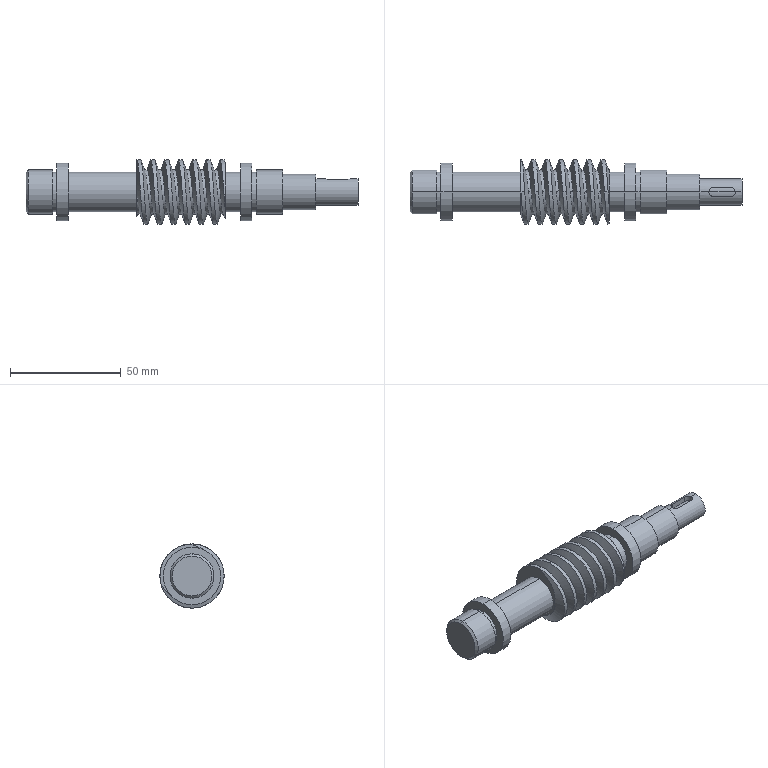Part | SolidWorks | features ICE 11, Chamfer 1, Extrusion 1, Helix 1, HoleWzd 1, SweepCut 1 | 1 solid | 76 faces | box 150 x 29 x 29 mm | volume 48060 mm3 | cylinder 52 | plane 14 | cone 6 | spline 4 | commonest cylinder face diameters 20 x18 29 x14 18 x8 12 x4 26 x4 4.2 x2